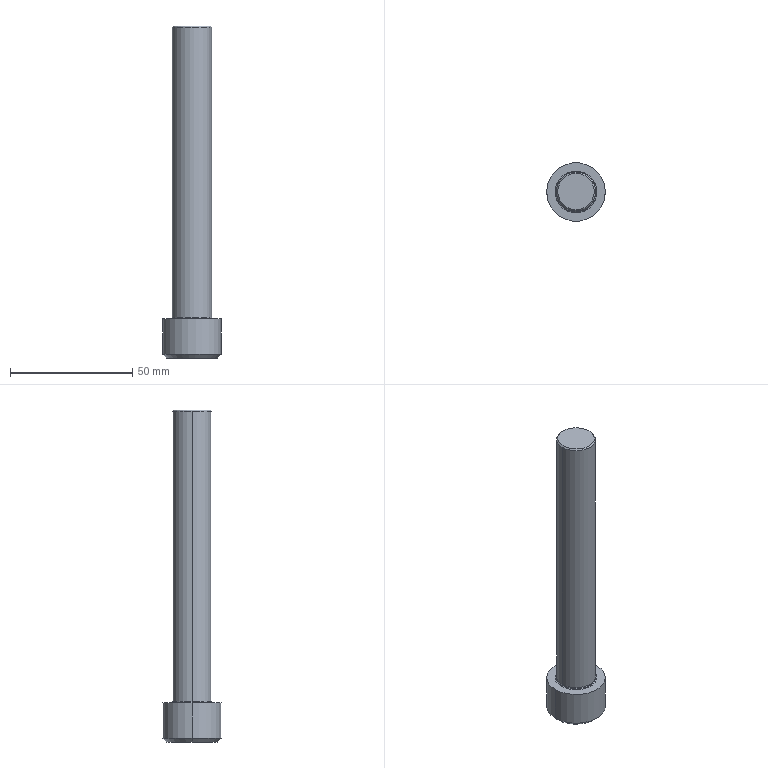Part | Creo | 1 solid | 23 faces | box 24 x 24 x 136 mm | volume 29603 mm3 | plane 9 | cone 6 | cylinder 4 | torus 4 | commonest cylinder face diameters 16 x2 24 x2
STEP:
#1=CARTESIAN_POINT('',(0.,0.,0.));
#2=DIRECTION('',(0.,0.,1.));
#3=DIRECTION('',(1.,0.,0.));
#4=AXIS2_PLACEMENT_3D('',#1,#2,#3);
#5=CARTESIAN_POINT('',(-178.083,120.,20.5));
#6=VERTEX_POINT('',#5);
#7=CARTESIAN_POINT('',(-174.041,127.,20.5));
#8=VERTEX_POINT('',#7);
#9=CARTESIAN_POINT('',(-178.083,120.,20.5));
#10=CARTESIAN_POINT('',(-177.863,120.381,20.627));
#11=CARTESIAN_POINT('',(-177.422,121.145,20.851));
#12=CARTESIAN_POINT('',(-176.746,122.315,21.073));
#13=CARTESIAN_POINT('',(-176.064,123.496,21.151));
#14=CARTESIAN_POINT('',(-175.379,124.683,21.073));
#15=CARTESIAN_POINT('',(-174.705,125.85,20.852));
#16=CARTESIAN_POINT('',(-174.262,126.618,20.627));
#17=CARTESIAN_POINT('',(-174.041,127.,20.5));
#18=B_SPLINE_CURVE_WITH_KNOTS('',3,(#9,#10,#11,#12,#13,#14,#15,#16,#17),.UNSPECIFIED.,.F.,.F.,(4,1,1,1,1,1,4),(0.,0.1667,0.3333,0.5,0.6667,0.8333,1.),.UNSPECIFIED.);
#19=EDGE_CURVE('',#6,#8,#18,.T.);
#20=ORIENTED_EDGE('',*,*,#19,.F.);
#21=CARTESIAN_POINT('',(-170.,120.,25.167));
#22=VERTEX_POINT('',#21);
#23=CARTESIAN_POINT('',(-170.,120.,25.167));
#24=DIRECTION('',(-0.866,0.,-0.5));
#25=VECTOR('',#24,9.333);
#26=LINE('',#23,#25);
#27=EDGE_CURVE('',#22,#6,#26,.T.);
#28=ORIENTED_EDGE('',*,*,#27,.F.);
#29=CARTESIAN_POINT('',(-161.917,120.,20.5));
#30=VERTEX_POINT('',#29);
#31=CARTESIAN_POINT('',(-170.,120.,25.167));
#32=DIRECTION('',(0.866,0.,-0.5));
#33=VECTOR('',#32,9.333);
#34=LINE('',#31,#33);
#35=EDGE_CURVE('',#22,#30,#34,.T.);
#36=ORIENTED_EDGE('',*,*,#35,.T.);
#37=CARTESIAN_POINT('',(-165.959,127.,20.5));
#38=VERTEX_POINT('',#37);
#39=CARTESIAN_POINT('',(-165.959,127.,20.5));
#40=CARTESIAN_POINT('',(-165.739,126.619,20.627));
#41=CARTESIAN_POINT('',(-165.297,125.855,20.851));
#42=CARTESIAN_POINT('',(-164.622,124.685,21.073));
#43=CARTESIAN_POINT('',(-163.94,123.504,21.151));
#44=CARTESIAN_POINT('',(-163.255,122.317,21.073));
#45=CARTESIAN_POINT('',(-162.581,121.15,20.852));
#46=CARTESIAN_POINT('',(-162.138,120.382,20.627));
#47=CARTESIAN_POINT('',(-161.917,120.,20.5));
#48=B_SPLINE_CURVE_WITH_KNOTS('',3,(#39,#40,#41,#42,#43,#44,#45,#46,#47),.UNSPECIFIED.,.F.,.F.,(4,1,1,1,1,1,4),(0.,0.1667,0.3333,0.5,0.6667,0.8333,1.),.UNSPECIFIED.);
#49=EDGE_CURVE('',#38,#30,#48,.T.);
#50=ORIENTED_EDGE('',*,*,#49,.F.);
#51=CARTESIAN_POINT('',(-174.041,127.,20.5));
#52=CARTESIAN_POINT('',(-173.604,127.,20.626));
#53=CARTESIAN_POINT('',(-172.723,127.,20.85));
#54=CARTESIAN_POINT('',(-171.369,127.,21.073));
#55=CARTESIAN_POINT('',(-170.002,127.,21.151));
#56=CARTESIAN_POINT('',(-168.637,127.,21.074));
#57=CARTESIAN_POINT('',(-167.283,127.,20.851));
#58=CARTESIAN_POINT('',(-166.399,127.,20.627));
#59=CARTESIAN_POINT('',(-165.959,127.,20.5));
#60=B_SPLINE_CURVE_WITH_KNOTS('',3,(#51,#52,#53,#54,#55,#56,#57,#58,#59),.UNSPECIFIED.,.F.,.F.,(4,1,1,1,1,1,4),(0.,0.1667,0.3333,0.5,0.6667,0.8333,1.),.UNSPECIFIED.);
#61=EDGE_CURVE('',#8,#38,#60,.T.);
#62=ORIENTED_EDGE('',*,*,#61,.F.);
#63=EDGE_LOOP('',(#20,#28,#36,#50,#62));
#64=FACE_OUTER_BOUND('',#63,.F.);
#65=CARTESIAN_POINT('',(-170.,120.,22.787));
#66=DIRECTION('',(0.,0.,-1.));
#67=DIRECTION('',(-1.,0.,0.));
#68=AXIS2_PLACEMENT_3D('',#65,#66,#67);
#69=CONICAL_SURFACE('',#68,4.122,60.);
#70=ADVANCED_FACE('',(#64),#69,.F.);
#71=CARTESIAN_POINT('',(-174.041,127.,12.5));
#72=VERTEX_POINT('',#71);
#73=CARTESIAN_POINT('',(-178.083,120.,12.5));
#74=VERTEX_POINT('',#73);
#75=CARTESIAN_POINT('',(-174.041,127.,12.5));
#76=DIRECTION('',(-0.5,-0.866,0.));
#77=VECTOR('',#76,8.083);
#78=LINE('',#75,#77);
#79=EDGE_CURVE('',#72,#74,#78,.T.);
#80=ORIENTED_EDGE('',*,*,#79,.T.);
#81=CARTESIAN_POINT('',(-178.083,120.,12.5));
#82=DIRECTION('',(0.,0.,1.));
#83=VECTOR('',#82,8.);
#84=LINE('',#81,#83);
#85=EDGE_CURVE('',#74,#6,#84,.T.);
#86=ORIENTED_EDGE('',*,*,#85,.T.);
#87=ORIENTED_EDGE('',*,*,#19,.T.);
#88=CARTESIAN_POINT('',(-174.041,127.,12.5));
#89=DIRECTION('',(0.,0.,1.));
#90=VECTOR('',#89,8.);
#91=LINE('',#88,#90);
#92=EDGE_CURVE('',#72,#8,#91,.T.);
#93=ORIENTED_EDGE('',*,*,#92,.F.);
#94=EDGE_LOOP('',(#80,#86,#87,#93));
#95=FACE_OUTER_BOUND('',#94,.F.);
#96=CARTESIAN_POINT('',(-174.041,127.,20.5));
#97=DIRECTION('',(0.866,-0.5,0.));
#98=DIRECTION('',(-0.5,-0.866,0.));
#99=AXIS2_PLACEMENT_3D('',#96,#97,#98);
#100=PLANE('',#99);
#101=ADVANCED_FACE('',(#95),#100,.T.);
#102=CARTESIAN_POINT('',(-180.4,120.,12.5));
#103=VERTEX_POINT('',#102);
#104=CARTESIAN_POINT('',(-159.6,120.,12.5));
#105=VERTEX_POINT('',#104);
#106=CARTESIAN_POINT('',(-170.,120.,12.5));
#107=DIRECTION('',(0.,0.,-1.));
#108=DIRECTION('',(-1.,0.,0.));
#109=AXIS2_PLACEMENT_3D('',#106,#107,#108);
#110=CIRCLE('',#109,10.4);
#111=EDGE_CURVE('',#103,#105,#110,.T.);
#112=ORIENTED_EDGE('',*,*,#111,.F.);
#113=CARTESIAN_POINT('',(-170.,120.,12.5));
#114=DIRECTION('',(0.,0.,-1.));
#115=DIRECTION('',(1.,0.,0.));
#116=AXIS2_PLACEMENT_3D('',#113,#114,#115);
#117=CIRCLE('',#116,10.4);
#118=EDGE_CURVE('',#105,#103,#117,.T.);
#119=ORIENTED_EDGE('',*,*,#118,.F.);
#120=EDGE_LOOP('',(#112,#119));
#121=FACE_OUTER_BOUND('',#120,.F.);
#122=CARTESIAN_POINT('',(-174.041,113.,12.5));
#123=VERTEX_POINT('',#122);
#124=CARTESIAN_POINT('',(-178.083,120.,12.5));
#125=DIRECTION('',(0.5,-0.866,0.));
#126=VECTOR('',#125,8.083);
#127=LINE('',#124,#126);
#128=EDGE_CURVE('',#74,#123,#127,.T.);
#129=ORIENTED_EDGE('',*,*,#128,.F.);
#130=ORIENTED_EDGE('',*,*,#79,.F.);
#131=CARTESIAN_POINT('',(-165.959,127.,12.5));
#132=VERTEX_POINT('',#131);
#133=CARTESIAN_POINT('',(-174.041,127.,12.5));
#134=DIRECTION('',(1.,0.,0.));
#135=VECTOR('',#134,8.083);
#136=LINE('',#133,#135);
#137=EDGE_CURVE('',#72,#132,#136,.T.);
#138=ORIENTED_EDGE('',*,*,#137,.T.);
#139=CARTESIAN_POINT('',(-161.917,120.,12.5));
#140=VERTEX_POINT('',#139);
#141=CARTESIAN_POINT('',(-161.917,120.,12.5));
#142=DIRECTION('',(-0.5,0.866,0.));
#143=VECTOR('',#142,8.083);
#144=LINE('',#141,#143);
#145=EDGE_CURVE('',#140,#132,#144,.T.);
#146=ORIENTED_EDGE('',*,*,#145,.F.);
#147=CARTESIAN_POINT('',(-165.959,113.,12.5));
#148=VERTEX_POINT('',#147);
#149=CARTESIAN_POINT('',(-165.959,113.,12.5));
#150=DIRECTION('',(0.5,0.866,0.));
#151=VECTOR('',#150,8.083);
#152=LINE('',#149,#151);
#153=EDGE_CURVE('',#148,#140,#152,.T.);
#154=ORIENTED_EDGE('',*,*,#153,.F.);
#155=CARTESIAN_POINT('',(-165.959,113.,12.5));
#156=DIRECTION('',(-1.,0.,0.));
#157=VECTOR('',#156,8.083);
#158=LINE('',#155,#157);
#159=EDGE_CURVE('',#148,#123,#158,.T.);
#160=ORIENTED_EDGE('',*,*,#159,.T.);
#161=EDGE_LOOP('',(#129,#130,#138,#146,#154,#160));
#162=FACE_BOUND('',#161,.F.);
#163=CARTESIAN_POINT('',(-170.,120.,12.5));
#164=DIRECTION('',(0.,0.,-1.));
#165=DIRECTION('',(-1.,0.,0.));
#166=AXIS2_PLACEMENT_3D('',#163,#164,#165);
#167=PLANE('',#166);
#168=ADVANCED_FACE('',(#121,#162),#167,.T.);
#169=CARTESIAN_POINT('',(-182.,120.,14.1));
#170=VERTEX_POINT('',#169);
#171=CARTESIAN_POINT('',(-158.,120.,14.1));
#172=VERTEX_POINT('',#171);
#173=CARTESIAN_POINT('',(-170.,120.,14.1));
#174=DIRECTION('',(0.,0.,-1.));
#175=DIRECTION('',(-1.,0.,0.));
#176=AXIS2_PLACEMENT_3D('',#173,#174,#175);
#177=CIRCLE('',#176,12.);
#178=EDGE_CURVE('',#170,#172,#177,.T.);
#179=ORIENTED_EDGE('',*,*,#178,.F.);
#180=CARTESIAN_POINT('',(-180.4,120.,12.5));
#181=DIRECTION('',(-0.7071,0.,0.7071));
#182=VECTOR('',#181,2.263);
#183=LINE('',#180,#182);
#184=EDGE_CURVE('',#103,#170,#183,.T.);
#185=ORIENTED_EDGE('',*,*,#184,.F.);
#186=ORIENTED_EDGE('',*,*,#111,.T.);
#187=CARTESIAN_POINT('',(-159.6,120.,12.5));
#188=DIRECTION('',(0.7071,0.,0.7071));
#189=VECTOR('',#188,2.263);
#190=LINE('',#187,#189);
#191=EDGE_CURVE('',#105,#172,#190,.T.);
#192=ORIENTED_EDGE('',*,*,#191,.T.);
#193=EDGE_LOOP('',(#179,#185,#186,#192));
#194=FACE_OUTER_BOUND('',#193,.F.);
#195=CARTESIAN_POINT('',(-170.,120.,13.3));
#196=DIRECTION('',(0.,0.,1.));
#197=DIRECTION('',(1.,0.,0.));
#198=AXIS2_PLACEMENT_3D('',#195,#196,#197);
#199=CONICAL_SURFACE('',#198,11.2,45.);
#200=ADVANCED_FACE('',(#194),#199,.T.);
#201=ORIENTED_EDGE('',*,*,#178,.T.);
#202=CARTESIAN_POINT('',(-158.,120.,28.5));
#203=VERTEX_POINT('',#202);
#204=CARTESIAN_POINT('',(-158.,120.,28.5));
#205=DIRECTION('',(0.,0.,-1.));
#206=VECTOR('',#205,14.4);
#207=LINE('',#204,#206);
#208=EDGE_CURVE('',#203,#172,#207,.T.);
#209=ORIENTED_EDGE('',*,*,#208,.F.);
#210=CARTESIAN_POINT('',(-182.,120.,28.5));
#211=VERTEX_POINT('',#210);
#212=CARTESIAN_POINT('',(-170.,120.,28.5));
#213=DIRECTION('',(0.,0.,1.));
#214=DIRECTION('',(1.,0.,0.));
#215=AXIS2_PLACEMENT_3D('',#212,#213,#214);
#216=CIRCLE('',#215,12.);
#217=EDGE_CURVE('',#203,#211,#216,.T.);
#218=ORIENTED_EDGE('',*,*,#217,.T.);
#219=CARTESIAN_POINT('',(-182.,120.,28.5));
#220=DIRECTION('',(0.,0.,-1.));
#221=VECTOR('',#220,14.4);
#222=LINE('',#219,#221);
#223=EDGE_CURVE('',#211,#170,#222,.T.);
#224=ORIENTED_EDGE('',*,*,#223,.T.);
#225=EDGE_LOOP('',(#201,#209,#218,#224));
#226=FACE_OUTER_BOUND('',#225,.F.);
#227=CARTESIAN_POINT('',(-170.,120.,28.5));
#228=DIRECTION('',(0.,0.,-1.));
#229=DIRECTION('',(-1.,0.,0.));
#230=AXIS2_PLACEMENT_3D('',#227,#228,#229);
#231=CYLINDRICAL_SURFACE('',#230,12.);
#232=ADVANCED_FACE('',(#226),#231,.T.);
#233=CARTESIAN_POINT('',(-170.,120.,14.1));
#234=DIRECTION('',(0.,0.,-1.));
#235=DIRECTION('',(1.,0.,0.));
#236=AXIS2_PLACEMENT_3D('',#233,#234,#235);
#237=CIRCLE('',#236,12.);
#238=EDGE_CURVE('',#172,#170,#237,.T.);
#239=ORIENTED_EDGE('',*,*,#238,.T.);
#240=ORIENTED_EDGE('',*,*,#223,.F.);
#241=CARTESIAN_POINT('',(-170.,120.,28.5));
#242=DIRECTION('',(0.,0.,1.));
#243=DIRECTION('',(-1.,0.,0.));
#244=AXIS2_PLACEMENT_3D('',#241,#242,#243);
#245=CIRCLE('',#244,12.);
#246=EDGE_CURVE('',#211,#203,#245,.T.);
#247=ORIENTED_EDGE('',*,*,#246,.T.);
#248=ORIENTED_EDGE('',*,*,#208,.T.);
#249=EDGE_LOOP('',(#239,#240,#247,#248));
#250=FACE_OUTER_BOUND('',#249,.F.);
#251=CARTESIAN_POINT('',(-170.,120.,28.5));
#252=DIRECTION('',(0.,0.,-1.));
#253=DIRECTION('',(-1.,0.,0.));
#254=AXIS2_PLACEMENT_3D('',#251,#252,#253);
#255=CYLINDRICAL_SURFACE('',#254,12.);
#256=ADVANCED_FACE('',(#250),#255,.T.);
#257=ORIENTED_EDGE('',*,*,#238,.F.);
#258=ORIENTED_EDGE('',*,*,#191,.F.);
#259=ORIENTED_EDGE('',*,*,#118,.T.);
#260=ORIENTED_EDGE('',*,*,#184,.T.);
#261=EDGE_LOOP('',(#257,#258,#259,#260));
#262=FACE_OUTER_BOUND('',#261,.F.);
#263=CARTESIAN_POINT('',(-170.,120.,13.3));
#264=DIRECTION('',(0.,0.,1.));
#265=DIRECTION('',(1.,0.,0.));
#266=AXIS2_PLACEMENT_3D('',#263,#264,#265);
#267=CONICAL_SURFACE('',#266,11.2,45.);
#268=ADVANCED_FACE('',(#262),#267,.T.);
#269=ORIENTED_EDGE('',*,*,#246,.F.);
#270=ORIENTED_EDGE('',*,*,#217,.F.);
#271=EDGE_LOOP('',(#269,#270));
#272=FACE_OUTER_BOUND('',#271,.F.);
#273=CARTESIAN_POINT('',(-178.6,120.,28.5));
#274=VERTEX_POINT('',#273);
#275=CARTESIAN_POINT('',(-161.4,120.,28.5));
#276=VERTEX_POINT('',#275);
#277=CARTESIAN_POINT('',(-170.,120.,28.5));
#278=DIRECTION('',(0.,0.,-1.));
#279=DIRECTION('',(-1.,0.,0.));
#280=AXIS2_PLACEMENT_3D('',#277,#278,#279);
#281=CIRCLE('',#280,8.6);
#282=EDGE_CURVE('',#274,#276,#281,.T.);
#283=ORIENTED_EDGE('',*,*,#282,.F.);
#284=CARTESIAN_POINT('',(-170.,120.,28.5));
#285=DIRECTION('',(0.,0.,-1.));
#286=DIRECTION('',(1.,0.,0.));
#287=AXIS2_PLACEMENT_3D('',#284,#285,#286);
#288=CIRCLE('',#287,8.6);
#289=EDGE_CURVE('',#276,#274,#288,.T.);
#290=ORIENTED_EDGE('',*,*,#289,.F.);
#291=EDGE_LOOP('',(#283,#290));
#292=FACE_BOUND('',#291,.F.);
#293=CARTESIAN_POINT('',(-170.,120.,28.5));
#294=DIRECTION('',(0.,0.,-1.));
#295=DIRECTION('',(-1.,0.,0.));
#296=AXIS2_PLACEMENT_3D('',#293,#294,#295);
#297=PLANE('',#296);
#298=ADVANCED_FACE('',(#272,#292),#297,.F.);
#299=ORIENTED_EDGE('',*,*,#282,.T.);
#300=CARTESIAN_POINT('',(-161.824,120.,28.676));
#301=VERTEX_POINT('',#300);
#302=CARTESIAN_POINT('',(-161.4,120.,29.1));
#303=DIRECTION('',(0.,1.,0.));
#304=DIRECTION('',(0.,0.,-1.));
#305=AXIS2_PLACEMENT_3D('',#302,#303,#304);
#306=CIRCLE('',#305,0.6);
#307=EDGE_CURVE('',#276,#301,#306,.T.);
#308=ORIENTED_EDGE('',*,*,#307,.T.);
#309=CARTESIAN_POINT('',(-178.176,120.,28.676));
#310=VERTEX_POINT('',#309);
#311=CARTESIAN_POINT('',(-170.,120.,28.676));
#312=DIRECTION('',(0.,0.,-1.));
#313=DIRECTION('',(-1.,0.,0.));
#314=AXIS2_PLACEMENT_3D('',#311,#312,#313);
#315=CIRCLE('',#314,8.176);
#316=EDGE_CURVE('',#310,#301,#315,.T.);
#317=ORIENTED_EDGE('',*,*,#316,.F.);
#318=CARTESIAN_POINT('',(-178.6,120.,29.1));
#319=DIRECTION('',(0.,-1.,0.));
#320=DIRECTION('',(0.,0.,-1.));
#321=AXIS2_PLACEMENT_3D('',#318,#319,#320);
#322=CIRCLE('',#321,0.6);
#323=EDGE_CURVE('',#274,#310,#322,.T.);
#324=ORIENTED_EDGE('',*,*,#323,.F.);
#325=EDGE_LOOP('',(#299,#308,#317,#324));
#326=FACE_OUTER_BOUND('',#325,.F.);
#327=CARTESIAN_POINT('',(-170.,120.,29.1));
#328=DIRECTION('',(0.,0.,-1.));
#329=DIRECTION('',(-1.,0.,0.));
#330=AXIS2_PLACEMENT_3D('',#327,#328,#329);
#331=TOROIDAL_SURFACE('',#330,8.6,0.6);
#332=ADVANCED_FACE('',(#326),#331,.F.);
#333=ORIENTED_EDGE('',*,*,#289,.T.);
#334=ORIENTED_EDGE('',*,*,#323,.T.);
#335=CARTESIAN_POINT('',(-170.,120.,28.676));
#336=DIRECTION('',(0.,0.,-1.));
#337=DIRECTION('',(1.,0.,0.));
#338=AXIS2_PLACEMENT_3D('',#335,#336,#337);
#339=CIRCLE('',#338,8.176);
#340=EDGE_CURVE('',#301,#310,#339,.T.);
#341=ORIENTED_EDGE('',*,*,#340,.F.);
#342=ORIENTED_EDGE('',*,*,#307,.F.);
#343=EDGE_LOOP('',(#333,#334,#341,#342));
#344=FACE_OUTER_BOUND('',#343,.F.);
#345=CARTESIAN_POINT('',(-170.,120.,29.1));
#346=DIRECTION('',(0.,0.,-1.));
#347=DIRECTION('',(-1.,0.,0.));
#348=AXIS2_PLACEMENT_3D('',#345,#346,#347);
#349=TOROIDAL_SURFACE('',#348,8.6,0.6);
#350=ADVANCED_FACE('',(#344),#349,.F.);
#351=CARTESIAN_POINT('',(-162.,120.,29.1));
#352=VERTEX_POINT('',#351);
#353=CARTESIAN_POINT('',(-178.,120.,29.1));
#354=VERTEX_POINT('',#353);
#355=CARTESIAN_POINT('',(-170.,120.,29.1));
#356=DIRECTION('',(0.,0.,-1.));
#357=DIRECTION('',(1.,0.,0.));
#358=AXIS2_PLACEMENT_3D('',#355,#356,#357);
#359=CIRCLE('',#358,8.);
#360=EDGE_CURVE('',#352,#354,#359,.T.);
#361=ORIENTED_EDGE('',*,*,#360,.F.);
#362=CARTESIAN_POINT('',(-161.4,120.,29.1));
#363=DIRECTION('',(0.,1.,0.));
#364=DIRECTION('',(-0.7071,0.,-0.7071));
#365=AXIS2_PLACEMENT_3D('',#362,#363,#364);
#366=CIRCLE('',#365,0.6);
#367=EDGE_CURVE('',#301,#352,#366,.T.);
#368=ORIENTED_EDGE('',*,*,#367,.F.);
#369=ORIENTED_EDGE('',*,*,#340,.T.);
#370=CARTESIAN_POINT('',(-178.6,120.,29.1));
#371=DIRECTION('',(0.,-1.,0.));
#372=DIRECTION('',(0.7071,0.,-0.7071));
#373=AXIS2_PLACEMENT_3D('',#370,#371,#372);
#374=CIRCLE('',#373,0.6);
#375=EDGE_CURVE('',#310,#354,#374,.T.);
#376=ORIENTED_EDGE('',*,*,#375,.T.);
#377=EDGE_LOOP('',(#361,#368,#369,#376));
#378=FACE_OUTER_BOUND('',#377,.F.);
#379=CARTESIAN_POINT('',(-170.,120.,29.1));
#380=DIRECTION('',(0.,0.,-1.));
#381=DIRECTION('',(-1.,0.,0.));
#382=AXIS2_PLACEMENT_3D('',#379,#380,#381);
#383=TOROIDAL_SURFACE('',#382,8.6,0.6);
#384=ADVANCED_FACE('',(#378),#383,.F.);
#385=CARTESIAN_POINT('',(-178.,120.,148.));
#386=VERTEX_POINT('',#385);
#387=CARTESIAN_POINT('',(-162.,120.,148.));
#388=VERTEX_POINT('',#387);
#389=CARTESIAN_POINT('',(-170.,120.,148.));
#390=DIRECTION('',(0.,0.,1.));
#391=DIRECTION('',(-1.,0.,0.));
#392=AXIS2_PLACEMENT_3D('',#389,#390,#391);
#393=CIRCLE('',#392,8.);
#394=EDGE_CURVE('',#386,#388,#393,.T.);
#395=ORIENTED_EDGE('',*,*,#394,.T.);
#396=CARTESIAN_POINT('',(-162.,120.,148.));
#397=DIRECTION('',(0.,0.,-1.));
#398=VECTOR('',#397,118.9);
#399=LINE('',#396,#398);
#400=EDGE_CURVE('',#388,#352,#399,.T.);
#401=ORIENTED_EDGE('',*,*,#400,.T.);
#402=ORIENTED_EDGE('',*,*,#360,.T.);
#403=CARTESIAN_POINT('',(-178.,120.,148.));
#404=DIRECTION('',(0.,0.,-1.));
#405=VECTOR('',#404,118.9);
#406=LINE('',#403,#405);
#407=EDGE_CURVE('',#386,#354,#406,.T.);
#408=ORIENTED_EDGE('',*,*,#407,.F.);
#409=EDGE_LOOP('',(#395,#401,#402,#408));
#410=FACE_OUTER_BOUND('',#409,.F.);
#411=CARTESIAN_POINT('',(-170.,120.,148.5));
#412=DIRECTION('',(0.,0.,-1.));
#413=DIRECTION('',(-1.,0.,0.));
#414=AXIS2_PLACEMENT_3D('',#411,#412,#413);
#415=CYLINDRICAL_SURFACE('',#414,8.);
#416=ADVANCED_FACE('',(#410),#415,.T.);
#417=CARTESIAN_POINT('',(-177.5,120.,148.5));
#418=VERTEX_POINT('',#417);
#419=CARTESIAN_POINT('',(-162.5,120.,148.5));
#420=VERTEX_POINT('',#419);
#421=CARTESIAN_POINT('',(-170.,120.,148.5));
#422=DIRECTION('',(0.,0.,1.));
#423=DIRECTION('',(-1.,0.,0.));
#424=AXIS2_PLACEMENT_3D('',#421,#422,#423);
#425=CIRCLE('',#424,7.5);
#426=EDGE_CURVE('',#418,#420,#425,.T.);
#427=ORIENTED_EDGE('',*,*,#426,.T.);
#428=CARTESIAN_POINT('',(-162.5,120.,148.5));
#429=DIRECTION('',(0.7071,0.,-0.7071));
#430=VECTOR('',#429,0.7071);
#431=LINE('',#428,#430);
#432=EDGE_CURVE('',#420,#388,#431,.T.);
#433=ORIENTED_EDGE('',*,*,#432,.T.);
#434=ORIENTED_EDGE('',*,*,#394,.F.);
#435=CARTESIAN_POINT('',(-177.5,120.,148.5));
#436=DIRECTION('',(-0.7071,0.,-0.7071));
#437=VECTOR('',#436,0.7071);
#438=LINE('',#435,#437);
#439=EDGE_CURVE('',#418,#386,#438,.T.);
#440=ORIENTED_EDGE('',*,*,#439,.F.);
#441=EDGE_LOOP('',(#427,#433,#434,#440));
#442=FACE_OUTER_BOUND('',#441,.F.);
#443=CARTESIAN_POINT('',(-170.,120.,148.25));
#444=DIRECTION('',(0.,0.,-1.));
#445=DIRECTION('',(-1.,0.,0.));
#446=AXIS2_PLACEMENT_3D('',#443,#444,#445);
#447=CONICAL_SURFACE('',#446,7.75,45.);
#448=ADVANCED_FACE('',(#442),#447,.T.);
#449=ORIENTED_EDGE('',*,*,#426,.F.);
#450=CARTESIAN_POINT('',(-170.,120.,148.5));
#451=DIRECTION('',(0.,0.,1.));
#452=DIRECTION('',(1.,0.,0.));
#453=AXIS2_PLACEMENT_3D('',#450,#451,#452);
#454=CIRCLE('',#453,7.5);
#455=EDGE_CURVE('',#420,#418,#454,.T.);
#456=ORIENTED_EDGE('',*,*,#455,.F.);
#457=EDGE_LOOP('',(#449,#456));
#458=FACE_OUTER_BOUND('',#457,.F.);
#459=CARTESIAN_POINT('',(-170.,120.,148.5));
#460=DIRECTION('',(0.,0.,-1.));
#461=DIRECTION('',(-1.,0.,0.));
#462=AXIS2_PLACEMENT_3D('',#459,#460,#461);
#463=PLANE('',#462);
#464=ADVANCED_FACE('',(#458),#463,.F.);
#465=ORIENTED_EDGE('',*,*,#455,.T.);
#466=ORIENTED_EDGE('',*,*,#439,.T.);
#467=CARTESIAN_POINT('',(-170.,120.,148.));
#468=DIRECTION('',(0.,0.,1.));
#469=DIRECTION('',(1.,0.,0.));
#470=AXIS2_PLACEMENT_3D('',#467,#468,#469);
#471=CIRCLE('',#470,8.);
#472=EDGE_CURVE('',#388,#386,#471,.T.);
#473=ORIENTED_EDGE('',*,*,#472,.F.);
#474=ORIENTED_EDGE('',*,*,#432,.F.);
#475=EDGE_LOOP('',(#465,#466,#473,#474));
#476=FACE_OUTER_BOUND('',#475,.F.);
#477=CARTESIAN_POINT('',(-170.,120.,148.25));
#478=DIRECTION('',(0.,0.,-1.));
#479=DIRECTION('',(-1.,0.,0.));
#480=AXIS2_PLACEMENT_3D('',#477,#478,#479);
#481=CONICAL_SURFACE('',#480,7.75,45.);
#482=ADVANCED_FACE('',(#476),#481,.T.);
#483=ORIENTED_EDGE('',*,*,#472,.T.);
#484=ORIENTED_EDGE('',*,*,#407,.T.);
#485=CARTESIAN_POINT('',(-170.,120.,29.1));
#486=DIRECTION('',(0.,0.,-1.));
#487=DIRECTION('',(-1.,0.,0.));
#488=AXIS2_PLACEMENT_3D('',#485,#486,#487);
#489=CIRCLE('',#488,8.);
#490=EDGE_CURVE('',#354,#352,#489,.T.);
#491=ORIENTED_EDGE('',*,*,#490,.T.);
#492=ORIENTED_EDGE('',*,*,#400,.F.);
#493=EDGE_LOOP('',(#483,#484,#491,#492));
#494=FACE_OUTER_BOUND('',#493,.F.);
#495=CARTESIAN_POINT('',(-170.,120.,148.5));
#496=DIRECTION('',(0.,0.,-1.));
#497=DIRECTION('',(-1.,0.,0.));
#498=AXIS2_PLACEMENT_3D('',#495,#496,#497);
#499=CYLINDRICAL_SURFACE('',#498,8.);
#500=ADVANCED_FACE('',(#494),#499,.T.);
#501=ORIENTED_EDGE('',*,*,#490,.F.);
#502=ORIENTED_EDGE('',*,*,#375,.F.);
#503=ORIENTED_EDGE('',*,*,#316,.T.);
#504=ORIENTED_EDGE('',*,*,#367,.T.);
#505=EDGE_LOOP('',(#501,#502,#503,#504));
#506=FACE_OUTER_BOUND('',#505,.F.);
#507=CARTESIAN_POINT('',(-170.,120.,29.1));
#508=DIRECTION('',(0.,0.,-1.));
#509=DIRECTION('',(-1.,0.,0.));
#510=AXIS2_PLACEMENT_3D('',#507,#508,#509);
#511=TOROIDAL_SURFACE('',#510,8.6,0.6);
#512=ADVANCED_FACE('',(#506),#511,.F.);
#513=ORIENTED_EDGE('',*,*,#128,.T.);
#514=CARTESIAN_POINT('',(-174.041,113.,20.5));
#515=VERTEX_POINT('',#514);
#516=CARTESIAN_POINT('',(-174.041,113.,12.5));
#517=DIRECTION('',(0.,0.,1.));
#518=VECTOR('',#517,8.);
#519=LINE('',#516,#518);
#520=EDGE_CURVE('',#123,#515,#519,.T.);
#521=ORIENTED_EDGE('',*,*,#520,.T.);
#522=CARTESIAN_POINT('',(-174.041,113.,20.5));
#523=CARTESIAN_POINT('',(-174.261,113.381,20.627));
#524=CARTESIAN_POINT('',(-174.703,114.145,20.851));
#525=CARTESIAN_POINT('',(-175.378,115.315,21.073));
#526=CARTESIAN_POINT('',(-176.06,116.496,21.151));
#527=CARTESIAN_POINT('',(-176.745,117.683,21.073));
#528=CARTESIAN_POINT('',(-177.419,118.85,20.852));
#529=CARTESIAN_POINT('',(-177.862,119.618,20.627));
#530=CARTESIAN_POINT('',(-178.083,120.,20.5));
#531=B_SPLINE_CURVE_WITH_KNOTS('',3,(#522,#523,#524,#525,#526,#527,#528,#529,#530),.UNSPECIFIED.,.F.,.F.,(4,1,1,1,1,1,4),(0.,0.1667,0.3333,0.5,0.6667,0.8333,1.),.UNSPECIFIED.);
#532=EDGE_CURVE('',#515,#6,#531,.T.);
#533=ORIENTED_EDGE('',*,*,#532,.T.);
#534=ORIENTED_EDGE('',*,*,#85,.F.);
#535=EDGE_LOOP('',(#513,#521,#533,#534));
#536=FACE_OUTER_BOUND('',#535,.F.);
#537=CARTESIAN_POINT('',(-178.083,120.,20.5));
#538=DIRECTION('',(0.866,0.5,0.));
#539=DIRECTION('',(0.5,-0.866,0.));
#540=AXIS2_PLACEMENT_3D('',#537,#538,#539);
#541=PLANE('',#540);
#542=ADVANCED_FACE('',(#536),#541,.T.);
#543=ORIENTED_EDGE('',*,*,#159,.F.);
#544=CARTESIAN_POINT('',(-165.959,113.,20.5));
#545=VERTEX_POINT('',#544);
#546=CARTESIAN_POINT('',(-165.959,113.,12.5));
#547=DIRECTION('',(0.,0.,1.));
#548=VECTOR('',#547,8.);
#549=LINE('',#546,#548);
#550=EDGE_CURVE('',#148,#545,#549,.T.);
#551=ORIENTED_EDGE('',*,*,#550,.T.);
#552=CARTESIAN_POINT('',(-165.959,113.,20.5));
#553=CARTESIAN_POINT('',(-166.399,113.,20.627));
#554=CARTESIAN_POINT('',(-167.283,113.,20.851));
#555=CARTESIAN_POINT('',(-168.637,113.,21.074));
#556=CARTESIAN_POINT('',(-170.002,113.,21.151));
#557=CARTESIAN_POINT('',(-171.369,113.,21.073));
#558=CARTESIAN_POINT('',(-172.723,113.,20.85));
#559=CARTESIAN_POINT('',(-173.604,113.,20.626));
#560=CARTESIAN_POINT('',(-174.041,113.,20.5));
#561=B_SPLINE_CURVE_WITH_KNOTS('',3,(#552,#553,#554,#555,#556,#557,#558,#559,#560),.UNSPECIFIED.,.F.,.F.,(4,1,1,1,1,1,4),(0.,0.1667,0.3333,0.5,0.6667,0.8333,1.),.UNSPECIFIED.);
#562=EDGE_CURVE('',#545,#515,#561,.T.);
#563=ORIENTED_EDGE('',*,*,#562,.T.);
#564=ORIENTED_EDGE('',*,*,#520,.F.);
#565=EDGE_LOOP('',(#543,#551,#563,#564));
#566=FACE_OUTER_BOUND('',#565,.F.);
#567=CARTESIAN_POINT('',(-174.041,113.,20.5));
#568=DIRECTION('',(0.,1.,0.));
#569=DIRECTION('',(0.,0.,-1.));
#570=AXIS2_PLACEMENT_3D('',#567,#568,#569);
#571=PLANE('',#570);
#572=ADVANCED_FACE('',(#566),#571,.T.);
#573=ORIENTED_EDGE('',*,*,#153,.T.);
#574=CARTESIAN_POINT('',(-161.917,120.,12.5));
#575=DIRECTION('',(0.,0.,1.));
#576=VECTOR('',#575,8.);
#577=LINE('',#574,#576);
#578=EDGE_CURVE('',#140,#30,#577,.T.);
#579=ORIENTED_EDGE('',*,*,#578,.T.);
#580=CARTESIAN_POINT('',(-161.917,120.,20.5));
#581=CARTESIAN_POINT('',(-162.138,119.618,20.627));
#582=CARTESIAN_POINT('',(-162.581,118.85,20.852));
#583=CARTESIAN_POINT('',(-163.255,117.683,21.073));
#584=CARTESIAN_POINT('',(-163.94,116.496,21.151));
#585=CARTESIAN_POINT('',(-164.622,115.315,21.073));
#586=CARTESIAN_POINT('',(-165.297,114.145,20.851));
#587=CARTESIAN_POINT('',(-165.739,113.381,20.627));
#588=CARTESIAN_POINT('',(-165.959,113.,20.5));
#589=B_SPLINE_CURVE_WITH_KNOTS('',3,(#580,#581,#582,#583,#584,#585,#586,#587,#588),.UNSPECIFIED.,.F.,.F.,(4,1,1,1,1,1,4),(0.,0.1667,0.3333,0.5,0.6667,0.8333,1.),.UNSPECIFIED.);
#590=EDGE_CURVE('',#30,#545,#589,.T.);
#591=ORIENTED_EDGE('',*,*,#590,.T.);
#592=ORIENTED_EDGE('',*,*,#550,.F.);
#593=EDGE_LOOP('',(#573,#579,#591,#592));
#594=FACE_OUTER_BOUND('',#593,.F.);
#595=CARTESIAN_POINT('',(-165.959,113.,20.5));
#596=DIRECTION('',(-0.866,0.5,0.));
#597=DIRECTION('',(0.5,0.866,0.));
#598=AXIS2_PLACEMENT_3D('',#595,#596,#597);
#599=PLANE('',#598);
#600=ADVANCED_FACE('',(#594),#599,.T.);
#601=ORIENTED_EDGE('',*,*,#145,.T.);
#602=CARTESIAN_POINT('',(-165.959,127.,12.5));
#603=DIRECTION('',(0.,0.,1.));
#604=VECTOR('',#603,8.);
#605=LINE('',#602,#604);
#606=EDGE_CURVE('',#132,#38,#605,.T.);
#607=ORIENTED_EDGE('',*,*,#606,.T.);
#608=ORIENTED_EDGE('',*,*,#49,.T.);
#609=ORIENTED_EDGE('',*,*,#578,.F.);
#610=EDGE_LOOP('',(#601,#607,#608,#609));
#611=FACE_OUTER_BOUND('',#610,.F.);
#612=CARTESIAN_POINT('',(-161.917,120.,20.5));
#613=DIRECTION('',(-0.866,-0.5,0.));
#614=DIRECTION('',(-0.5,0.866,0.));
#615=AXIS2_PLACEMENT_3D('',#612,#613,#614);
#616=PLANE('',#615);
#617=ADVANCED_FACE('',(#611),#616,.T.);
#618=ORIENTED_EDGE('',*,*,#137,.F.);
#619=ORIENTED_EDGE('',*,*,#92,.T.);
#620=ORIENTED_EDGE('',*,*,#61,.T.);
#621=ORIENTED_EDGE('',*,*,#606,.F.);
#622=EDGE_LOOP('',(#618,#619,#620,#621));
#623=FACE_OUTER_BOUND('',#622,.F.);
#624=CARTESIAN_POINT('',(-165.959,127.,20.5));
#625=DIRECTION('',(0.,-1.,0.));
#626=DIRECTION('',(0.,0.,1.));
#627=AXIS2_PLACEMENT_3D('',#624,#625,#626);
#628=PLANE('',#627);
#629=ADVANCED_FACE('',(#623),#628,.T.);
#630=ORIENTED_EDGE('',*,*,#590,.F.);
#631=ORIENTED_EDGE('',*,*,#35,.F.);
#632=ORIENTED_EDGE('',*,*,#27,.T.);
#633=ORIENTED_EDGE('',*,*,#532,.F.);
#634=ORIENTED_EDGE('',*,*,#562,.F.);
#635=EDGE_LOOP('',(#630,#631,#632,#633,#634));
#636=FACE_OUTER_BOUND('',#635,.F.);
#637=CARTESIAN_POINT('',(-170.,120.,22.787));
#638=DIRECTION('',(0.,0.,-1.));
#639=DIRECTION('',(-1.,0.,0.));
#640=AXIS2_PLACEMENT_3D('',#637,#638,#639);
#641=CONICAL_SURFACE('',#640,4.122,60.);
#642=ADVANCED_FACE('',(#636),#641,.F.);
#643=CLOSED_SHELL('',(#70,#101,#168,#200,#232,#256,#268,#298,#332,#350,#384,#416,#448,#464,#482,#500,#512,#542,#572,#600,#617,#629,#642));
#644=MANIFOLD_SOLID_BREP('',#643);
#645=(LENGTH_UNIT()NAMED_UNIT(*)SI_UNIT(.MILLI.,.METRE.));
#646=UNCERTAINTY_MEASURE_WITH_UNIT(LENGTH_MEASURE(0.01402),#645,'','');
#647=(NAMED_UNIT(*)PLANE_ANGLE_UNIT()SI_UNIT($,.RADIAN.));
#648=PLANE_ANGLE_MEASURE_WITH_UNIT(PLANE_ANGLE_MEASURE(0.01745),#647);
#649=(CONVERSION_BASED_UNIT('DEGREE',#648)NAMED_UNIT(*)PLANE_ANGLE_UNIT());
#650=(NAMED_UNIT(*)SI_UNIT($,.STERADIAN.)SOLID_ANGLE_UNIT());
#651=(GEOMETRIC_REPRESENTATION_CONTEXT(3)GLOBAL_UNCERTAINTY_ASSIGNED_CONTEXT((#646))GLOBAL_UNIT_ASSIGNED_CONTEXT((#645,#649,#650))REPRESENTATION_CONTEXT('',''));
#652=ADVANCED_BREP_SHAPE_REPRESENTATION('',(#4,#644),#651);